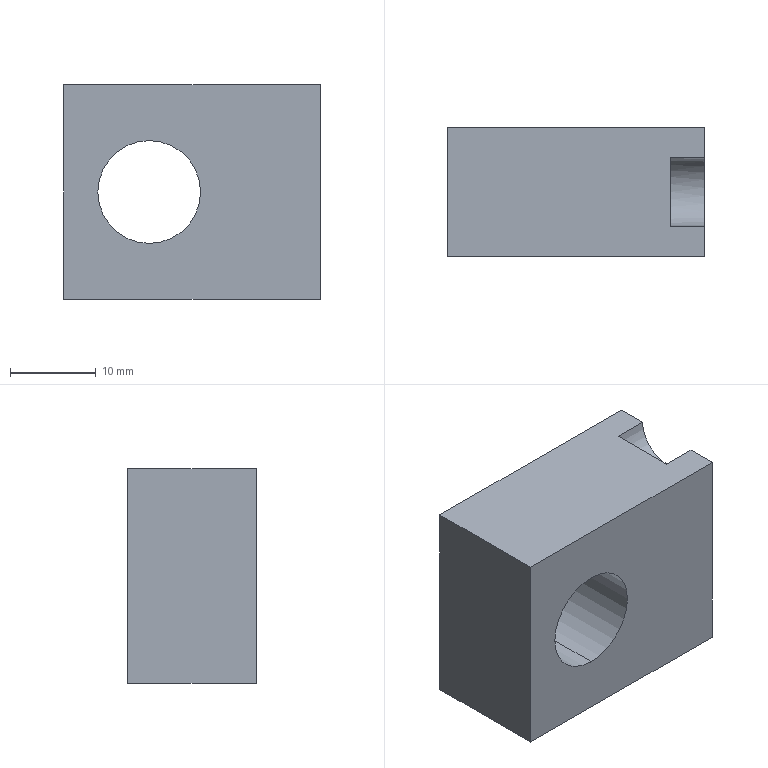Part | STEP file | Positioning_id1606_x_t | 1 solid | 13 faces | box 30 x 15 x 25 mm | volume 9340 mm3 | plane 8 | cylinder 5 | commonest cylinder face diameters 6 x2 12 x2 8 x1
STEP:
#1=CARTESIAN_POINT('',(0.,0.,0.));
#2=DIRECTION('',(0.,0.,1.));
#3=DIRECTION('',(1.,0.,0.));
#4=AXIS2_PLACEMENT_3D('',#1,#2,#3);
#5=CARTESIAN_POINT('',(-751.002,-201.5,188.032));
#6=VERTEX_POINT('',#5);
#7=CARTESIAN_POINT('',(-751.002,-201.5,194.032));
#8=VERTEX_POINT('',#7);
#9=CARTESIAN_POINT('',(-751.002,-201.5,191.032));
#10=DIRECTION('',(1.,0.,0.));
#11=DIRECTION('',(0.,0.,-1.));
#12=AXIS2_PLACEMENT_3D('',#9,#10,#11);
#13=CIRCLE('',#12,3.);
#14=CARTESIAN_POINT('',(-701.002,-201.5,191.032));
#15=DIRECTION('',(1.,0.,0.));
#16=DIRECTION('',(0.,0.,-1.));
#17=AXIS2_PLACEMENT_3D('',#14,#15,#16);
#18=CYLINDRICAL_SURFACE('',#17,3.);
#19=CARTESIAN_POINT('',(0.,-50.));
#20=DIRECTION('',(1.,0.));
#21=VECTOR('',#20,1.);
#22=LINE('',#19,#21);
#23=(GEOMETRIC_REPRESENTATION_CONTEXT(2)PARAMETRIC_REPRESENTATION_CONTEXT()REPRESENTATION_CONTEXT('',''));
#24=DEFINITIONAL_REPRESENTATION('',(#22),#23);
#25=PCURVE('',#18,#24);
#26=CARTESIAN_POINT('',(-751.002,-201.5,191.032));
#27=DIRECTION('',(-1.,0.,0.));
#28=DIRECTION('',(0.,0.,-1.));
#29=AXIS2_PLACEMENT_3D('',#26,#27,#28);
#30=PLANE('',#29);
#31=CARTESIAN_POINT('',(3.,0.));
#32=CARTESIAN_POINT('',(3.,-5.196));
#33=CARTESIAN_POINT('',(-1.5,-2.598));
#34=CARTESIAN_POINT('',(-6.,0.));
#35=CARTESIAN_POINT('',(-1.5,2.598));
#36=CARTESIAN_POINT('',(3.,5.196));
#37=CARTESIAN_POINT('',(3.,0.));
#38=(BOUNDED_CURVE()B_SPLINE_CURVE(2,(#31,#32,#33,#34,#35,#36,#37),.UNSPECIFIED.,.T.,.F.)B_SPLINE_CURVE_WITH_KNOTS((1,2,2,2,2,1),(-2.094,0.,2.094,4.189,6.283,8.378),.UNSPECIFIED.)CURVE()GEOMETRIC_REPRESENTATION_ITEM()RATIONAL_B_SPLINE_CURVE((1.,0.5,1.,0.5,1.,0.5,1.))REPRESENTATION_ITEM(''));
#39=(GEOMETRIC_REPRESENTATION_CONTEXT(2)PARAMETRIC_REPRESENTATION_CONTEXT()REPRESENTATION_CONTEXT('',''));
#40=DEFINITIONAL_REPRESENTATION('',(#38),#39);
#41=PCURVE('',#30,#40);
#42=SURFACE_CURVE('',#13,(#25,#41),.PCURVE_S1.);
#43=EDGE_CURVE('',#6,#8,#42,.T.);
#44=ORIENTED_EDGE('',*,*,#43,.T.);
#45=CARTESIAN_POINT('',(-747.002,-201.5,194.032));
#46=VERTEX_POINT('',#45);
#47=CARTESIAN_POINT('',(-747.002,-201.5,194.032));
#48=DIRECTION('',(1.,0.,0.));
#49=VECTOR('',#48,1.);
#50=LINE('',#47,#49);
#51=CARTESIAN_POINT('',(3.142,-46.));
#52=DIRECTION('',(0.,1.));
#53=VECTOR('',#52,1.);
#54=LINE('',#51,#53);
#55=(GEOMETRIC_REPRESENTATION_CONTEXT(2)PARAMETRIC_REPRESENTATION_CONTEXT()REPRESENTATION_CONTEXT('',''));
#56=DEFINITIONAL_REPRESENTATION('',(#54),#55);
#57=PCURVE('',#18,#56);
#58=CARTESIAN_POINT('',(-701.002,-201.5,191.032));
#59=DIRECTION('',(1.,0.,0.));
#60=DIRECTION('',(0.,0.,-1.));
#61=AXIS2_PLACEMENT_3D('',#58,#59,#60);
#62=CYLINDRICAL_SURFACE('',#61,3.);
#63=CARTESIAN_POINT('',(3.142,-46.));
#64=DIRECTION('',(0.,1.));
#65=VECTOR('',#64,1.);
#66=LINE('',#63,#65);
#67=(GEOMETRIC_REPRESENTATION_CONTEXT(2)PARAMETRIC_REPRESENTATION_CONTEXT()REPRESENTATION_CONTEXT('',''));
#68=DEFINITIONAL_REPRESENTATION('',(#66),#67);
#69=PCURVE('',#62,#68);
#70=SURFACE_CURVE('',#50,(#57,#69),.PCURVE_S1.);
#71=EDGE_CURVE('',#8,#46,#70,.T.);
#72=ORIENTED_EDGE('',*,*,#71,.T.);
#73=CARTESIAN_POINT('',(-747.002,-201.5,188.032));
#74=VERTEX_POINT('',#73);
#75=CARTESIAN_POINT('',(-747.002,-201.5,191.032));
#76=DIRECTION('',(-1.,0.,0.));
#77=DIRECTION('',(0.,0.,-1.));
#78=AXIS2_PLACEMENT_3D('',#75,#76,#77);
#79=CIRCLE('',#78,3.);
#80=CARTESIAN_POINT('',(6.283,-46.));
#81=DIRECTION('',(-1.,0.));
#82=VECTOR('',#81,1.);
#83=LINE('',#80,#82);
#84=(GEOMETRIC_REPRESENTATION_CONTEXT(2)PARAMETRIC_REPRESENTATION_CONTEXT()REPRESENTATION_CONTEXT('',''));
#85=DEFINITIONAL_REPRESENTATION('',(#83),#84);
#86=PCURVE('',#18,#85);
#87=CARTESIAN_POINT('',(-747.002,-194.,206.032));
#88=DIRECTION('',(1.,0.,0.));
#89=DIRECTION('',(0.,0.,-1.));
#90=AXIS2_PLACEMENT_3D('',#87,#88,#89);
#91=PLANE('',#90);
#92=CARTESIAN_POINT('',(18.,-7.5));
#93=CARTESIAN_POINT('',(18.,-12.696));
#94=CARTESIAN_POINT('',(13.5,-10.098));
#95=CARTESIAN_POINT('',(9.,-7.5));
#96=CARTESIAN_POINT('',(13.5,-4.902));
#97=CARTESIAN_POINT('',(18.,-2.304));
#98=CARTESIAN_POINT('',(18.,-7.5));
#99=(BOUNDED_CURVE()B_SPLINE_CURVE(2,(#92,#93,#94,#95,#96,#97,#98),.UNSPECIFIED.,.T.,.F.)B_SPLINE_CURVE_WITH_KNOTS((1,2,2,2,2,1),(-2.094,0.,2.094,4.189,6.283,8.378),.UNSPECIFIED.)CURVE()GEOMETRIC_REPRESENTATION_ITEM()RATIONAL_B_SPLINE_CURVE((1.,0.5,1.,0.5,1.,0.5,1.))REPRESENTATION_ITEM(''));
#100=(GEOMETRIC_REPRESENTATION_CONTEXT(2)PARAMETRIC_REPRESENTATION_CONTEXT()REPRESENTATION_CONTEXT('',''));
#101=DEFINITIONAL_REPRESENTATION('',(#99),#100);
#102=PCURVE('',#91,#101);
#103=SURFACE_CURVE('',#79,(#86,#102),.PCURVE_S1.);
#104=EDGE_CURVE('',#46,#74,#103,.T.);
#105=ORIENTED_EDGE('',*,*,#104,.T.);
#106=CARTESIAN_POINT('',(-747.002,-201.5,188.032));
#107=DIRECTION('',(-1.,0.,0.));
#108=VECTOR('',#107,1.);
#109=LINE('',#106,#108);
#110=CARTESIAN_POINT('',(0.,-46.));
#111=DIRECTION('',(0.,-1.));
#112=VECTOR('',#111,1.);
#113=LINE('',#110,#112);
#114=(GEOMETRIC_REPRESENTATION_CONTEXT(2)PARAMETRIC_REPRESENTATION_CONTEXT()REPRESENTATION_CONTEXT('',''));
#115=DEFINITIONAL_REPRESENTATION('',(#113),#114);
#116=PCURVE('',#18,#115);
#117=CARTESIAN_POINT('',(6.283,-46.));
#118=DIRECTION('',(0.,-1.));
#119=VECTOR('',#118,1.);
#120=LINE('',#117,#119);
#121=(GEOMETRIC_REPRESENTATION_CONTEXT(2)PARAMETRIC_REPRESENTATION_CONTEXT()REPRESENTATION_CONTEXT('',''));
#122=DEFINITIONAL_REPRESENTATION('',(#120),#121);
#123=PCURVE('',#62,#122);
#124=SURFACE_CURVE('',#109,(#116,#123),.PCURVE_S1.);
#125=EDGE_CURVE('',#74,#6,#124,.T.);
#126=ORIENTED_EDGE('',*,*,#125,.T.);
#127=EDGE_LOOP('',(#44,#72,#105,#126));
#128=FACE_BOUND('',#127,.F.);
#129=ADVANCED_FACE('',(#128),#18,.F.);
#130=CARTESIAN_POINT('',(-751.002,-201.5,194.032));
#131=CARTESIAN_POINT('',(-751.002,-204.5,194.032));
#132=CARTESIAN_POINT('',(-751.002,-206.,191.032));
#133=CARTESIAN_POINT('',(-751.002,-204.5,188.032));
#134=CARTESIAN_POINT('',(-751.002,-201.5,188.032));
#135=(BOUNDED_CURVE()B_SPLINE_CURVE(4,(#130,#131,#132,#133,#134),.UNSPECIFIED.,.F.,.F.)B_SPLINE_CURVE_WITH_KNOTS((5,5),(0.,1.),.PIECEWISE_BEZIER_KNOTS.)CURVE()GEOMETRIC_REPRESENTATION_ITEM()RATIONAL_B_SPLINE_CURVE((1.,0.7071,0.6667,0.7071,1.))REPRESENTATION_ITEM(''));
#136=CARTESIAN_POINT('',(-3.,0.));
#137=CARTESIAN_POINT('',(-3.,3.));
#138=CARTESIAN_POINT('',(0.,4.5));
#139=CARTESIAN_POINT('',(3.,3.));
#140=CARTESIAN_POINT('',(3.,0.));
#141=(BOUNDED_CURVE()B_SPLINE_CURVE(4,(#136,#137,#138,#139,#140),.UNSPECIFIED.,.F.,.F.)B_SPLINE_CURVE_WITH_KNOTS((5,5),(0.,1.),.PIECEWISE_BEZIER_KNOTS.)CURVE()GEOMETRIC_REPRESENTATION_ITEM()RATIONAL_B_SPLINE_CURVE((1.,0.7071,0.6667,0.7071,1.))REPRESENTATION_ITEM(''));
#142=(GEOMETRIC_REPRESENTATION_CONTEXT(2)PARAMETRIC_REPRESENTATION_CONTEXT()REPRESENTATION_CONTEXT('',''));
#143=DEFINITIONAL_REPRESENTATION('',(#141),#142);
#144=PCURVE('',#30,#143);
#145=CARTESIAN_POINT('',(3.142,-50.));
#146=CARTESIAN_POINT('',(3.184,-50.));
#147=CARTESIAN_POINT('',(3.271,-50.));
#148=CARTESIAN_POINT('',(3.405,-50.));
#149=CARTESIAN_POINT('',(3.542,-50.));
#150=CARTESIAN_POINT('',(3.681,-50.));
#151=CARTESIAN_POINT('',(3.823,-50.));
#152=CARTESIAN_POINT('',(3.968,-50.));
#153=CARTESIAN_POINT('',(4.114,-50.));
#154=CARTESIAN_POINT('',(4.262,-50.));
#155=CARTESIAN_POINT('',(4.412,-50.));
#156=CARTESIAN_POINT('',(4.562,-50.));
#157=CARTESIAN_POINT('',(4.712,-50.));
#158=CARTESIAN_POINT('',(4.863,-50.));
#159=CARTESIAN_POINT('',(5.013,-50.));
#160=CARTESIAN_POINT('',(5.163,-50.));
#161=CARTESIAN_POINT('',(5.311,-50.));
#162=CARTESIAN_POINT('',(5.457,-50.));
#163=CARTESIAN_POINT('',(5.602,-50.));
#164=CARTESIAN_POINT('',(5.744,-50.));
#165=CARTESIAN_POINT('',(5.883,-50.));
#166=CARTESIAN_POINT('',(6.02,-50.));
#167=CARTESIAN_POINT('',(6.153,-50.));
#168=CARTESIAN_POINT('',(6.24,-50.));
#169=CARTESIAN_POINT('',(6.283,-50.));
#170=B_SPLINE_CURVE_WITH_KNOTS('',3,(#145,#146,#147,#148,#149,#150,#151,#152,#153,#154,#155,#156,#157,#158,#159,#160,#161,#162,#163,#164,#165,#166,#167,#168,#169),.UNSPECIFIED.,.F.,.F.,(4,1,1,1,1,1,1,1,1,1,1,1,1,1,1,1,1,1,1,1,1,1,4),(0.,0.04545,0.09091,0.1364,0.1818,0.2273,0.2727,0.3182,0.3636,0.4091,0.4545,0.5,0.5455,0.5909,0.6364,0.6818,0.7273,0.7727,0.8182,0.8636,0.9091,0.9545,1.),.QUASI_UNIFORM_KNOTS.);
#171=(GEOMETRIC_REPRESENTATION_CONTEXT(2)PARAMETRIC_REPRESENTATION_CONTEXT()REPRESENTATION_CONTEXT('',''));
#172=DEFINITIONAL_REPRESENTATION('',(#170),#171);
#173=PCURVE('',#62,#172);
#174=SURFACE_CURVE('',#135,(#144,#173),.PCURVE_S1.);
#175=EDGE_CURVE('',#8,#6,#174,.T.);
#176=ORIENTED_EDGE('',*,*,#175,.T.);
#177=ORIENTED_EDGE('',*,*,#43,.T.);
#178=EDGE_LOOP('',(#176,#177));
#179=FACE_BOUND('',#178,.T.);
#180=ADVANCED_FACE('',(#179),#30,.F.);
#181=CARTESIAN_POINT('',(-747.002,-194.,181.032));
#182=VERTEX_POINT('',#181);
#183=CARTESIAN_POINT('',(-777.002,-194.,181.032));
#184=VERTEX_POINT('',#183);
#185=CARTESIAN_POINT('',(-747.002,-194.,181.032));
#186=DIRECTION('',(-1.,0.,0.));
#187=VECTOR('',#186,1.);
#188=LINE('',#185,#187);
#189=CARTESIAN_POINT('',(-701.002,-191.5,181.032));
#190=DIRECTION('',(0.,0.,-1.));
#191=DIRECTION('',(0.,1.,0.));
#192=AXIS2_PLACEMENT_3D('',#189,#190,#191);
#193=PLANE('',#192);
#194=CARTESIAN_POINT('',(-2.5,-46.));
#195=DIRECTION('',(0.,-1.));
#196=VECTOR('',#195,1.);
#197=LINE('',#194,#196);
#198=(GEOMETRIC_REPRESENTATION_CONTEXT(2)PARAMETRIC_REPRESENTATION_CONTEXT()REPRESENTATION_CONTEXT('',''));
#199=DEFINITIONAL_REPRESENTATION('',(#197),#198);
#200=PCURVE('',#193,#199);
#201=CARTESIAN_POINT('',(-759.502,-194.,187.282));
#202=DIRECTION('',(0.,1.,0.));
#203=DIRECTION('',(1.,0.,0.));
#204=AXIS2_PLACEMENT_3D('',#201,#202,#203);
#205=PLANE('',#204);
#206=CARTESIAN_POINT('',(12.5,6.25));
#207=DIRECTION('',(-1.,0.));
#208=VECTOR('',#207,1.);
#209=LINE('',#206,#208);
#210=(GEOMETRIC_REPRESENTATION_CONTEXT(2)PARAMETRIC_REPRESENTATION_CONTEXT()REPRESENTATION_CONTEXT('',''));
#211=DEFINITIONAL_REPRESENTATION('',(#209),#210);
#212=PCURVE('',#205,#211);
#213=SURFACE_CURVE('',#188,(#200,#212),.PCURVE_S1.);
#214=EDGE_CURVE('',#182,#184,#213,.T.);
#215=ORIENTED_EDGE('',*,*,#214,.F.);
#216=CARTESIAN_POINT('',(-747.002,-209.,181.032));
#217=VERTEX_POINT('',#216);
#218=CARTESIAN_POINT('',(-747.002,-194.,181.032));
#219=DIRECTION('',(0.,-1.,0.));
#220=VECTOR('',#219,1.);
#221=LINE('',#218,#220);
#222=CARTESIAN_POINT('',(-2.5,-46.));
#223=DIRECTION('',(-1.,0.));
#224=VECTOR('',#223,1.);
#225=LINE('',#222,#224);
#226=(GEOMETRIC_REPRESENTATION_CONTEXT(2)PARAMETRIC_REPRESENTATION_CONTEXT()REPRESENTATION_CONTEXT('',''));
#227=DEFINITIONAL_REPRESENTATION('',(#225),#226);
#228=PCURVE('',#193,#227);
#229=CARTESIAN_POINT('',(25.,0.));
#230=DIRECTION('',(0.,-1.));
#231=VECTOR('',#230,1.);
#232=LINE('',#229,#231);
#233=(GEOMETRIC_REPRESENTATION_CONTEXT(2)PARAMETRIC_REPRESENTATION_CONTEXT()REPRESENTATION_CONTEXT('',''));
#234=DEFINITIONAL_REPRESENTATION('',(#232),#233);
#235=PCURVE('',#91,#234);
#236=SURFACE_CURVE('',#221,(#228,#235),.PCURVE_S1.);
#237=EDGE_CURVE('',#182,#217,#236,.T.);
#238=ORIENTED_EDGE('',*,*,#237,.T.);
#239=CARTESIAN_POINT('',(-777.002,-209.,181.032));
#240=VERTEX_POINT('',#239);
#241=CARTESIAN_POINT('',(-777.002,-209.,181.032));
#242=DIRECTION('',(1.,0.,0.));
#243=VECTOR('',#242,1.);
#244=LINE('',#241,#243);
#245=CARTESIAN_POINT('',(-17.5,-76.));
#246=DIRECTION('',(0.,1.));
#247=VECTOR('',#246,1.);
#248=LINE('',#245,#247);
#249=(GEOMETRIC_REPRESENTATION_CONTEXT(2)PARAMETRIC_REPRESENTATION_CONTEXT()REPRESENTATION_CONTEXT('',''));
#250=DEFINITIONAL_REPRESENTATION('',(#248),#249);
#251=PCURVE('',#193,#250);
#252=CARTESIAN_POINT('',(-759.502,-209.,187.282));
#253=DIRECTION('',(0.,-1.,0.));
#254=DIRECTION('',(-1.,0.,0.));
#255=AXIS2_PLACEMENT_3D('',#252,#253,#254);
#256=PLANE('',#255);
#257=CARTESIAN_POINT('',(17.5,6.25));
#258=DIRECTION('',(-1.,0.));
#259=VECTOR('',#258,1.);
#260=LINE('',#257,#259);
#261=(GEOMETRIC_REPRESENTATION_CONTEXT(2)PARAMETRIC_REPRESENTATION_CONTEXT()REPRESENTATION_CONTEXT('',''));
#262=DEFINITIONAL_REPRESENTATION('',(#260),#261);
#263=PCURVE('',#256,#262);
#264=SURFACE_CURVE('',#244,(#251,#263),.PCURVE_S1.);
#265=EDGE_CURVE('',#240,#217,#264,.T.);
#266=ORIENTED_EDGE('',*,*,#265,.F.);
#267=CARTESIAN_POINT('',(-777.002,-194.,181.032));
#268=DIRECTION('',(0.,-1.,0.));
#269=VECTOR('',#268,1.);
#270=LINE('',#267,#269);
#271=CARTESIAN_POINT('',(-2.5,-76.));
#272=DIRECTION('',(-1.,0.));
#273=VECTOR('',#272,1.);
#274=LINE('',#271,#273);
#275=(GEOMETRIC_REPRESENTATION_CONTEXT(2)PARAMETRIC_REPRESENTATION_CONTEXT()REPRESENTATION_CONTEXT('',''));
#276=DEFINITIONAL_REPRESENTATION('',(#274),#275);
#277=PCURVE('',#193,#276);
#278=CARTESIAN_POINT('',(-777.002,-201.5,187.282));
#279=DIRECTION('',(-1.,0.,0.));
#280=DIRECTION('',(0.,1.,0.));
#281=AXIS2_PLACEMENT_3D('',#278,#279,#280);
#282=PLANE('',#281);
#283=CARTESIAN_POINT('',(7.5,6.25));
#284=DIRECTION('',(-1.,0.));
#285=VECTOR('',#284,1.);
#286=LINE('',#283,#285);
#287=(GEOMETRIC_REPRESENTATION_CONTEXT(2)PARAMETRIC_REPRESENTATION_CONTEXT()REPRESENTATION_CONTEXT('',''));
#288=DEFINITIONAL_REPRESENTATION('',(#286),#287);
#289=PCURVE('',#282,#288);
#290=SURFACE_CURVE('',#270,(#277,#289),.PCURVE_S1.);
#291=EDGE_CURVE('',#184,#240,#290,.T.);
#292=ORIENTED_EDGE('',*,*,#291,.F.);
#293=EDGE_LOOP('',(#215,#238,#266,#292));
#294=FACE_BOUND('',#293,.T.);
#295=ADVANCED_FACE('',(#294),#193,.T.);
#296=CARTESIAN_POINT('',(-767.002,-209.,187.532));
#297=VERTEX_POINT('',#296);
#298=CARTESIAN_POINT('',(-767.002,-209.,199.532));
#299=VERTEX_POINT('',#298);
#300=CARTESIAN_POINT('',(-767.002,-209.,193.532));
#301=DIRECTION('',(0.,1.,0.));
#302=DIRECTION('',(0.,0.,-1.));
#303=AXIS2_PLACEMENT_3D('',#300,#301,#302);
#304=CIRCLE('',#303,6.);
#305=CARTESIAN_POINT('',(7.5,-0.25));
#306=CARTESIAN_POINT('',(17.892,-0.25));
#307=CARTESIAN_POINT('',(12.696,-9.25));
#308=CARTESIAN_POINT('',(7.5,-18.25));
#309=CARTESIAN_POINT('',(2.304,-9.25));
#310=CARTESIAN_POINT('',(-2.892,-0.25));
#311=CARTESIAN_POINT('',(7.5,-0.25));
#312=(BOUNDED_CURVE()B_SPLINE_CURVE(2,(#305,#306,#307,#308,#309,#310,#311),.UNSPECIFIED.,.T.,.F.)B_SPLINE_CURVE_WITH_KNOTS((1,2,2,2,2,1),(-2.094,0.,2.094,4.189,6.283,8.378),.UNSPECIFIED.)CURVE()GEOMETRIC_REPRESENTATION_ITEM()RATIONAL_B_SPLINE_CURVE((1.,0.5,1.,0.5,1.,0.5,1.))REPRESENTATION_ITEM(''));
#313=(GEOMETRIC_REPRESENTATION_CONTEXT(2)PARAMETRIC_REPRESENTATION_CONTEXT()REPRESENTATION_CONTEXT('',''));
#314=DEFINITIONAL_REPRESENTATION('',(#312),#313);
#315=PCURVE('',#256,#314);
#316=CARTESIAN_POINT('',(-767.002,-214.,193.532));
#317=DIRECTION('',(0.,-1.,0.));
#318=DIRECTION('',(0.,0.,1.));
#319=AXIS2_PLACEMENT_3D('',#316,#317,#318);
#320=CYLINDRICAL_SURFACE('',#319,6.);
#321=CARTESIAN_POINT('',(3.142,-5.));
#322=DIRECTION('',(-1.,0.));
#323=VECTOR('',#322,1.);
#324=LINE('',#321,#323);
#325=(GEOMETRIC_REPRESENTATION_CONTEXT(2)PARAMETRIC_REPRESENTATION_CONTEXT()REPRESENTATION_CONTEXT('',''));
#326=DEFINITIONAL_REPRESENTATION('',(#324),#325);
#327=PCURVE('',#320,#326);
#328=SURFACE_CURVE('',#304,(#315,#327),.PCURVE_S1.);
#329=EDGE_CURVE('',#297,#299,#328,.T.);
#330=ORIENTED_EDGE('',*,*,#329,.T.);
#331=CARTESIAN_POINT('',(-767.002,-209.,193.532));
#332=DIRECTION('',(0.,1.,0.));
#333=DIRECTION('',(0.,0.,1.));
#334=AXIS2_PLACEMENT_3D('',#331,#332,#333);
#335=CIRCLE('',#334,6.);
#336=CARTESIAN_POINT('',(7.5,-12.25));
#337=CARTESIAN_POINT('',(-2.892,-12.25));
#338=CARTESIAN_POINT('',(2.304,-3.25));
#339=CARTESIAN_POINT('',(7.5,5.75));
#340=CARTESIAN_POINT('',(12.696,-3.25));
#341=CARTESIAN_POINT('',(17.892,-12.25));
#342=CARTESIAN_POINT('',(7.5,-12.25));
#343=(BOUNDED_CURVE()B_SPLINE_CURVE(2,(#336,#337,#338,#339,#340,#341,#342),.UNSPECIFIED.,.T.,.F.)B_SPLINE_CURVE_WITH_KNOTS((1,2,2,2,2,1),(-2.094,0.,2.094,4.189,6.283,8.378),.UNSPECIFIED.)CURVE()GEOMETRIC_REPRESENTATION_ITEM()RATIONAL_B_SPLINE_CURVE((1.,0.5,1.,0.5,1.,0.5,1.))REPRESENTATION_ITEM(''));
#344=(GEOMETRIC_REPRESENTATION_CONTEXT(2)PARAMETRIC_REPRESENTATION_CONTEXT()REPRESENTATION_CONTEXT('',''));
#345=DEFINITIONAL_REPRESENTATION('',(#343),#344);
#346=PCURVE('',#256,#345);
#347=CARTESIAN_POINT('',(-767.002,-214.,193.532));
#348=DIRECTION('',(0.,-1.,0.));
#349=DIRECTION('',(0.,0.,1.));
#350=AXIS2_PLACEMENT_3D('',#347,#348,#349);
#351=CYLINDRICAL_SURFACE('',#350,6.);
#352=CARTESIAN_POINT('',(6.283,-5.));
#353=DIRECTION('',(-1.,0.));
#354=VECTOR('',#353,1.);
#355=LINE('',#352,#354);
#356=(GEOMETRIC_REPRESENTATION_CONTEXT(2)PARAMETRIC_REPRESENTATION_CONTEXT()REPRESENTATION_CONTEXT('',''));
#357=DEFINITIONAL_REPRESENTATION('',(#355),#356);
#358=PCURVE('',#351,#357);
#359=SURFACE_CURVE('',#335,(#346,#358),.PCURVE_S1.);
#360=EDGE_CURVE('',#299,#297,#359,.T.);
#361=ORIENTED_EDGE('',*,*,#360,.T.);
#362=EDGE_LOOP('',(#330,#361));
#363=FACE_BOUND('',#362,.T.);
#364=CARTESIAN_POINT('',(-747.002,-209.,206.032));
#365=VERTEX_POINT('',#364);
#366=CARTESIAN_POINT('',(-777.002,-209.,206.032));
#367=VERTEX_POINT('',#366);
#368=CARTESIAN_POINT('',(-747.002,-209.,206.032));
#369=DIRECTION('',(-1.,0.,0.));
#370=VECTOR('',#369,1.);
#371=LINE('',#368,#370);
#372=CARTESIAN_POINT('',(-12.5,-18.75));
#373=DIRECTION('',(1.,0.));
#374=VECTOR('',#373,1.);
#375=LINE('',#372,#374);
#376=(GEOMETRIC_REPRESENTATION_CONTEXT(2)PARAMETRIC_REPRESENTATION_CONTEXT()REPRESENTATION_CONTEXT('',''));
#377=DEFINITIONAL_REPRESENTATION('',(#375),#376);
#378=PCURVE('',#256,#377);
#379=CARTESIAN_POINT('',(-759.502,-201.5,206.032));
#380=DIRECTION('',(0.,0.,1.));
#381=DIRECTION('',(0.,-1.,0.));
#382=AXIS2_PLACEMENT_3D('',#379,#380,#381);
#383=PLANE('',#382);
#384=CARTESIAN_POINT('',(7.5,12.5));
#385=DIRECTION('',(0.,-1.));
#386=VECTOR('',#385,1.);
#387=LINE('',#384,#386);
#388=(GEOMETRIC_REPRESENTATION_CONTEXT(2)PARAMETRIC_REPRESENTATION_CONTEXT()REPRESENTATION_CONTEXT('',''));
#389=DEFINITIONAL_REPRESENTATION('',(#387),#388);
#390=PCURVE('',#383,#389);
#391=SURFACE_CURVE('',#371,(#378,#390),.PCURVE_S1.);
#392=EDGE_CURVE('',#365,#367,#391,.T.);
#393=ORIENTED_EDGE('',*,*,#392,.T.);
#394=CARTESIAN_POINT('',(-777.002,-209.,206.032));
#395=DIRECTION('',(0.,0.,-1.));
#396=VECTOR('',#395,1.);
#397=LINE('',#394,#396);
#398=CARTESIAN_POINT('',(17.5,-18.75));
#399=DIRECTION('',(0.,1.));
#400=VECTOR('',#399,1.);
#401=LINE('',#398,#400);
#402=(GEOMETRIC_REPRESENTATION_CONTEXT(2)PARAMETRIC_REPRESENTATION_CONTEXT()REPRESENTATION_CONTEXT('',''));
#403=DEFINITIONAL_REPRESENTATION('',(#401),#402);
#404=PCURVE('',#256,#403);
#405=CARTESIAN_POINT('',(-7.5,-18.75));
#406=DIRECTION('',(0.,1.));
#407=VECTOR('',#406,1.);
#408=LINE('',#405,#407);
#409=(GEOMETRIC_REPRESENTATION_CONTEXT(2)PARAMETRIC_REPRESENTATION_CONTEXT()REPRESENTATION_CONTEXT('',''));
#410=DEFINITIONAL_REPRESENTATION('',(#408),#409);
#411=PCURVE('',#282,#410);
#412=SURFACE_CURVE('',#397,(#404,#411),.PCURVE_S1.);
#413=EDGE_CURVE('',#367,#240,#412,.T.);
#414=ORIENTED_EDGE('',*,*,#413,.T.);
#415=ORIENTED_EDGE('',*,*,#265,.T.);
#416=CARTESIAN_POINT('',(-747.002,-209.,181.032));
#417=DIRECTION('',(0.,0.,1.));
#418=VECTOR('',#417,1.);
#419=LINE('',#416,#418);
#420=CARTESIAN_POINT('',(-12.5,6.25));
#421=DIRECTION('',(0.,-1.));
#422=VECTOR('',#421,1.);
#423=LINE('',#420,#422);
#424=(GEOMETRIC_REPRESENTATION_CONTEXT(2)PARAMETRIC_REPRESENTATION_CONTEXT()REPRESENTATION_CONTEXT('',''));
#425=DEFINITIONAL_REPRESENTATION('',(#423),#424);
#426=PCURVE('',#256,#425);
#427=CARTESIAN_POINT('',(25.,-15.));
#428=DIRECTION('',(-1.,0.));
#429=VECTOR('',#428,1.);
#430=LINE('',#427,#429);
#431=(GEOMETRIC_REPRESENTATION_CONTEXT(2)PARAMETRIC_REPRESENTATION_CONTEXT()REPRESENTATION_CONTEXT('',''));
#432=DEFINITIONAL_REPRESENTATION('',(#430),#431);
#433=PCURVE('',#91,#432);
#434=SURFACE_CURVE('',#419,(#426,#433),.PCURVE_S1.);
#435=EDGE_CURVE('',#217,#365,#434,.T.);
#436=ORIENTED_EDGE('',*,*,#435,.T.);
#437=EDGE_LOOP('',(#393,#414,#415,#436));
#438=FACE_BOUND('',#437,.T.);
#439=ADVANCED_FACE('',(#363,#438),#256,.T.);
#440=CARTESIAN_POINT('',(-747.002,-197.5,206.032));
#441=VERTEX_POINT('',#440);
#442=CARTESIAN_POINT('',(-751.002,-197.5,206.032));
#443=VERTEX_POINT('',#442);
#444=CARTESIAN_POINT('',(-747.002,-197.5,206.032));
#445=DIRECTION('',(-1.,0.,0.));
#446=VECTOR('',#445,1.);
#447=LINE('',#444,#446);
#448=CARTESIAN_POINT('',(-4.,12.5));
#449=DIRECTION('',(0.,-1.));
#450=VECTOR('',#449,1.);
#451=LINE('',#448,#450);
#452=(GEOMETRIC_REPRESENTATION_CONTEXT(2)PARAMETRIC_REPRESENTATION_CONTEXT()REPRESENTATION_CONTEXT('',''));
#453=DEFINITIONAL_REPRESENTATION('',(#451),#452);
#454=PCURVE('',#383,#453);
#455=CARTESIAN_POINT('',(-701.002,-201.5,206.032));
#456=DIRECTION('',(1.,0.,0.));
#457=DIRECTION('',(0.,0.,-1.));
#458=AXIS2_PLACEMENT_3D('',#455,#456,#457);
#459=CYLINDRICAL_SURFACE('',#458,4.);
#460=CARTESIAN_POINT('',(7.854,-46.));
#461=DIRECTION('',(0.,-1.));
#462=VECTOR('',#461,1.);
#463=LINE('',#460,#462);
#464=(GEOMETRIC_REPRESENTATION_CONTEXT(2)PARAMETRIC_REPRESENTATION_CONTEXT()REPRESENTATION_CONTEXT('',''));
#465=DEFINITIONAL_REPRESENTATION('',(#463),#464);
#466=PCURVE('',#459,#465);
#467=SURFACE_CURVE('',#447,(#454,#466),.PCURVE_S1.);
#468=EDGE_CURVE('',#441,#443,#467,.T.);
#469=ORIENTED_EDGE('',*,*,#468,.F.);
#470=CARTESIAN_POINT('',(-747.002,-194.,206.032));
#471=VERTEX_POINT('',#470);
#472=CARTESIAN_POINT('',(-747.002,-194.,206.032));
#473=DIRECTION('',(0.,-1.,0.));
#474=VECTOR('',#473,1.);
#475=LINE('',#472,#474);
#476=CARTESIAN_POINT('',(-7.5,12.5));
#477=DIRECTION('',(1.,0.));
#478=VECTOR('',#477,1.);
#479=LINE('',#476,#478);
#480=(GEOMETRIC_REPRESENTATION_CONTEXT(2)PARAMETRIC_REPRESENTATION_CONTEXT()REPRESENTATION_CONTEXT('',''));
#481=DEFINITIONAL_REPRESENTATION('',(#479),#480);
#482=PCURVE('',#383,#481);
#483=CARTESIAN_POINT('',(0.,0.));
#484=DIRECTION('',(0.,-1.));
#485=VECTOR('',#484,1.);
#486=LINE('',#483,#485);
#487=(GEOMETRIC_REPRESENTATION_CONTEXT(2)PARAMETRIC_REPRESENTATION_CONTEXT()REPRESENTATION_CONTEXT('',''));
#488=DEFINITIONAL_REPRESENTATION('',(#486),#487);
#489=PCURVE('',#91,#488);
#490=SURFACE_CURVE('',#475,(#482,#489),.PCURVE_S1.);
#491=EDGE_CURVE('',#471,#441,#490,.T.);
#492=ORIENTED_EDGE('',*,*,#491,.F.);
#493=CARTESIAN_POINT('',(-777.002,-194.,206.032));
#494=VERTEX_POINT('',#493);
#495=CARTESIAN_POINT('',(-777.002,-194.,206.032));
#496=DIRECTION('',(1.,0.,0.));
#497=VECTOR('',#496,1.);
#498=LINE('',#495,#497);
#499=CARTESIAN_POINT('',(-7.5,-17.5));
#500=DIRECTION('',(0.,1.));
#501=VECTOR('',#500,1.);
#502=LINE('',#499,#501);
#503=(GEOMETRIC_REPRESENTATION_CONTEXT(2)PARAMETRIC_REPRESENTATION_CONTEXT()REPRESENTATION_CONTEXT('',''));
#504=DEFINITIONAL_REPRESENTATION('',(#502),#503);
#505=PCURVE('',#383,#504);
#506=CARTESIAN_POINT('',(-17.5,-18.75));
#507=DIRECTION('',(1.,0.));
#508=VECTOR('',#507,1.);
#509=LINE('',#506,#508);
#510=(GEOMETRIC_REPRESENTATION_CONTEXT(2)PARAMETRIC_REPRESENTATION_CONTEXT()REPRESENTATION_CONTEXT('',''));
#511=DEFINITIONAL_REPRESENTATION('',(#509),#510);
#512=PCURVE('',#205,#511);
#513=SURFACE_CURVE('',#498,(#505,#512),.PCURVE_S1.);
#514=EDGE_CURVE('',#494,#471,#513,.T.);
#515=ORIENTED_EDGE('',*,*,#514,.F.);
#516=CARTESIAN_POINT('',(-777.002,-194.,206.032));
#517=DIRECTION('',(0.,-1.,0.));
#518=VECTOR('',#517,1.);
#519=LINE('',#516,#518);
#520=CARTESIAN_POINT('',(-7.5,-17.5));
#521=DIRECTION('',(1.,0.));
#522=VECTOR('',#521,1.);
#523=LINE('',#520,#522);
#524=(GEOMETRIC_REPRESENTATION_CONTEXT(2)PARAMETRIC_REPRESENTATION_CONTEXT()REPRESENTATION_CONTEXT('',''));
#525=DEFINITIONAL_REPRESENTATION('',(#523),#524);
#526=PCURVE('',#383,#525);
#527=CARTESIAN_POINT('',(7.5,-18.75));
#528=DIRECTION('',(-1.,0.));
#529=VECTOR('',#528,1.);
#530=LINE('',#527,#529);
#531=(GEOMETRIC_REPRESENTATION_CONTEXT(2)PARAMETRIC_REPRESENTATION_CONTEXT()REPRESENTATION_CONTEXT('',''));
#532=DEFINITIONAL_REPRESENTATION('',(#530),#531);
#533=PCURVE('',#282,#532);
#534=SURFACE_CURVE('',#519,(#526,#533),.PCURVE_S1.);
#535=EDGE_CURVE('',#494,#367,#534,.T.);
#536=ORIENTED_EDGE('',*,*,#535,.T.);
#537=ORIENTED_EDGE('',*,*,#392,.F.);
#538=CARTESIAN_POINT('',(-747.002,-205.5,206.032));
#539=VERTEX_POINT('',#538);
#540=CARTESIAN_POINT('',(-747.002,-205.5,206.032));
#541=DIRECTION('',(0.,-1.,0.));
#542=VECTOR('',#541,1.);
#543=LINE('',#540,#542);
#544=CARTESIAN_POINT('',(4.,12.5));
#545=DIRECTION('',(1.,0.));
#546=VECTOR('',#545,1.);
#547=LINE('',#544,#546);
#548=(GEOMETRIC_REPRESENTATION_CONTEXT(2)PARAMETRIC_REPRESENTATION_CONTEXT()REPRESENTATION_CONTEXT('',''));
#549=DEFINITIONAL_REPRESENTATION('',(#547),#548);
#550=PCURVE('',#383,#549);
#551=CARTESIAN_POINT('',(0.,-11.5));
#552=DIRECTION('',(0.,-1.));
#553=VECTOR('',#552,1.);
#554=LINE('',#551,#553);
#555=(GEOMETRIC_REPRESENTATION_CONTEXT(2)PARAMETRIC_REPRESENTATION_CONTEXT()REPRESENTATION_CONTEXT('',''));
#556=DEFINITIONAL_REPRESENTATION('',(#554),#555);
#557=PCURVE('',#91,#556);
#558=SURFACE_CURVE('',#543,(#550,#557),.PCURVE_S1.);
#559=EDGE_CURVE('',#539,#365,#558,.T.);
#560=ORIENTED_EDGE('',*,*,#559,.F.);
#561=CARTESIAN_POINT('',(-751.002,-205.5,206.032));
#562=VERTEX_POINT('',#561);
#563=CARTESIAN_POINT('',(-751.002,-205.5,206.032));
#564=DIRECTION('',(1.,0.,0.));
#565=VECTOR('',#564,1.);
#566=LINE('',#563,#565);
#567=CARTESIAN_POINT('',(4.,8.5));
#568=DIRECTION('',(0.,1.));
#569=VECTOR('',#568,1.);
#570=LINE('',#567,#569);
#571=(GEOMETRIC_REPRESENTATION_CONTEXT(2)PARAMETRIC_REPRESENTATION_CONTEXT()REPRESENTATION_CONTEXT('',''));
#572=DEFINITIONAL_REPRESENTATION('',(#570),#571);
#573=PCURVE('',#383,#572);
#574=CARTESIAN_POINT('',(4.712,-50.));
#575=DIRECTION('',(0.,1.));
#576=VECTOR('',#575,1.);
#577=LINE('',#574,#576);
#578=(GEOMETRIC_REPRESENTATION_CONTEXT(2)PARAMETRIC_REPRESENTATION_CONTEXT()REPRESENTATION_CONTEXT('',''));
#579=DEFINITIONAL_REPRESENTATION('',(#577),#578);
#580=PCURVE('',#459,#579);
#581=SURFACE_CURVE('',#566,(#573,#580),.PCURVE_S1.);
#582=EDGE_CURVE('',#562,#539,#581,.T.);
#583=ORIENTED_EDGE('',*,*,#582,.F.);
#584=CARTESIAN_POINT('',(-751.002,-197.5,206.032));
#585=DIRECTION('',(0.,-1.,0.));
#586=VECTOR('',#585,1.);
#587=LINE('',#584,#586);
#588=CARTESIAN_POINT('',(-4.,8.5));
#589=DIRECTION('',(1.,0.));
#590=VECTOR('',#589,1.);
#591=LINE('',#588,#590);
#592=(GEOMETRIC_REPRESENTATION_CONTEXT(2)PARAMETRIC_REPRESENTATION_CONTEXT()REPRESENTATION_CONTEXT('',''));
#593=DEFINITIONAL_REPRESENTATION('',(#591),#592);
#594=PCURVE('',#383,#593);
#595=CARTESIAN_POINT('',(-751.002,-201.5,206.032));
#596=DIRECTION('',(-1.,0.,0.));
#597=DIRECTION('',(0.,0.,-1.));
#598=AXIS2_PLACEMENT_3D('',#595,#596,#597);
#599=PLANE('',#598);
#600=CARTESIAN_POINT('',(0.,-4.));
#601=DIRECTION('',(0.,1.));
#602=VECTOR('',#601,1.);
#603=LINE('',#600,#602);
#604=(GEOMETRIC_REPRESENTATION_CONTEXT(2)PARAMETRIC_REPRESENTATION_CONTEXT()REPRESENTATION_CONTEXT('',''));
#605=DEFINITIONAL_REPRESENTATION('',(#603),#604);
#606=PCURVE('',#599,#605);
#607=SURFACE_CURVE('',#587,(#594,#606),.PCURVE_S1.);
#608=EDGE_CURVE('',#443,#562,#607,.T.);
#609=ORIENTED_EDGE('',*,*,#608,.F.);
#610=EDGE_LOOP('',(#469,#492,#515,#536,#537,#560,#583,#609));
#611=FACE_BOUND('',#610,.T.);
#612=ADVANCED_FACE('',(#611),#383,.T.);
#613=ORIENTED_EDGE('',*,*,#582,.F.);
#614=CARTESIAN_POINT('',(-751.002,-201.5,202.032));
#615=VERTEX_POINT('',#614);
#616=CARTESIAN_POINT('',(-751.002,-201.5,206.032));
#617=DIRECTION('',(1.,0.,0.));
#618=DIRECTION('',(0.,0.,-1.));
#619=AXIS2_PLACEMENT_3D('',#616,#617,#618);
#620=CIRCLE('',#619,4.);
#621=CARTESIAN_POINT('',(0.,-50.));
#622=DIRECTION('',(1.,0.));
#623=VECTOR('',#622,1.);
#624=LINE('',#621,#623);
#625=(GEOMETRIC_REPRESENTATION_CONTEXT(2)PARAMETRIC_REPRESENTATION_CONTEXT()REPRESENTATION_CONTEXT('',''));
#626=DEFINITIONAL_REPRESENTATION('',(#624),#625);
#627=PCURVE('',#459,#626);
#628=CARTESIAN_POINT('',(4.,0.));
#629=CARTESIAN_POINT('',(4.,-6.928));
#630=CARTESIAN_POINT('',(-2.,-3.464));
#631=CARTESIAN_POINT('',(-8.,0.));
#632=CARTESIAN_POINT('',(-2.,3.464));
#633=CARTESIAN_POINT('',(4.,6.928));
#634=CARTESIAN_POINT('',(4.,0.));
#635=(BOUNDED_CURVE()B_SPLINE_CURVE(2,(#628,#629,#630,#631,#632,#633,#634),.UNSPECIFIED.,.T.,.F.)B_SPLINE_CURVE_WITH_KNOTS((1,2,2,2,2,1),(-2.094,0.,2.094,4.189,6.283,8.378),.UNSPECIFIED.)CURVE()GEOMETRIC_REPRESENTATION_ITEM()RATIONAL_B_SPLINE_CURVE((1.,0.5,1.,0.5,1.,0.5,1.))REPRESENTATION_ITEM(''));
#636=(GEOMETRIC_REPRESENTATION_CONTEXT(2)PARAMETRIC_REPRESENTATION_CONTEXT()REPRESENTATION_CONTEXT('',''));
#637=DEFINITIONAL_REPRESENTATION('',(#635),#636);
#638=PCURVE('',#599,#637);
#639=SURFACE_CURVE('',#620,(#627,#638),.PCURVE_S1.);
#640=EDGE_CURVE('',#562,#615,#639,.T.);
#641=ORIENTED_EDGE('',*,*,#640,.T.);
#642=CARTESIAN_POINT('',(-751.002,-201.5,206.032));
#643=DIRECTION('',(1.,0.,0.));
#644=DIRECTION('',(0.,0.,-1.));
#645=AXIS2_PLACEMENT_3D('',#642,#643,#644);
#646=CIRCLE('',#645,4.);
#647=CARTESIAN_POINT('',(6.283,-50.));
#648=DIRECTION('',(1.,0.));
#649=VECTOR('',#648,1.);
#650=LINE('',#647,#649);
#651=(GEOMETRIC_REPRESENTATION_CONTEXT(2)PARAMETRIC_REPRESENTATION_CONTEXT()REPRESENTATION_CONTEXT('',''));
#652=DEFINITIONAL_REPRESENTATION('',(#650),#651);
#653=PCURVE('',#459,#652);
#654=CARTESIAN_POINT('',(4.,0.));
#655=CARTESIAN_POINT('',(4.,-6.928));
#656=CARTESIAN_POINT('',(-2.,-3.464));
#657=CARTESIAN_POINT('',(-8.,0.));
#658=CARTESIAN_POINT('',(-2.,3.464));
#659=CARTESIAN_POINT('',(4.,6.928));
#660=CARTESIAN_POINT('',(4.,0.));
#661=(BOUNDED_CURVE()B_SPLINE_CURVE(2,(#654,#655,#656,#657,#658,#659,#660),.UNSPECIFIED.,.T.,.F.)B_SPLINE_CURVE_WITH_KNOTS((1,2,2,2,2,1),(-2.094,0.,2.094,4.189,6.283,8.378),.UNSPECIFIED.)CURVE()GEOMETRIC_REPRESENTATION_ITEM()RATIONAL_B_SPLINE_CURVE((1.,0.5,1.,0.5,1.,0.5,1.))REPRESENTATION_ITEM(''));
#662=(GEOMETRIC_REPRESENTATION_CONTEXT(2)PARAMETRIC_REPRESENTATION_CONTEXT()REPRESENTATION_CONTEXT('',''));
#663=DEFINITIONAL_REPRESENTATION('',(#661),#662);
#664=PCURVE('',#599,#663);
#665=SURFACE_CURVE('',#646,(#653,#664),.PCURVE_S1.);
#666=EDGE_CURVE('',#615,#443,#665,.T.);
#667=ORIENTED_EDGE('',*,*,#666,.T.);
#668=ORIENTED_EDGE('',*,*,#468,.F.);
#669=CARTESIAN_POINT('',(-747.002,-201.5,206.032));
#670=DIRECTION('',(-1.,0.,0.));
#671=DIRECTION('',(0.,0.,-1.));
#672=AXIS2_PLACEMENT_3D('',#669,#670,#671);
#673=CIRCLE('',#672,4.);
#674=CARTESIAN_POINT('',(12.566,-46.));
#675=DIRECTION('',(-1.,0.));
#676=VECTOR('',#675,1.);
#677=LINE('',#674,#676);
#678=(GEOMETRIC_REPRESENTATION_CONTEXT(2)PARAMETRIC_REPRESENTATION_CONTEXT()REPRESENTATION_CONTEXT('',''));
#679=DEFINITIONAL_REPRESENTATION('',(#677),#678);
#680=PCURVE('',#459,#679);
#681=CARTESIAN_POINT('',(4.,-7.5));
#682=CARTESIAN_POINT('',(4.,-14.428));
#683=CARTESIAN_POINT('',(-2.,-10.964));
#684=CARTESIAN_POINT('',(-8.,-7.5));
#685=CARTESIAN_POINT('',(-2.,-4.036));
#686=CARTESIAN_POINT('',(4.,-0.5718));
#687=CARTESIAN_POINT('',(4.,-7.5));
#688=(BOUNDED_CURVE()B_SPLINE_CURVE(2,(#681,#682,#683,#684,#685,#686,#687),.UNSPECIFIED.,.T.,.F.)B_SPLINE_CURVE_WITH_KNOTS((1,2,2,2,2,1),(-2.094,0.,2.094,4.189,6.283,8.378),.UNSPECIFIED.)CURVE()GEOMETRIC_REPRESENTATION_ITEM()RATIONAL_B_SPLINE_CURVE((1.,0.5,1.,0.5,1.,0.5,1.))REPRESENTATION_ITEM(''));
#689=(GEOMETRIC_REPRESENTATION_CONTEXT(2)PARAMETRIC_REPRESENTATION_CONTEXT()REPRESENTATION_CONTEXT('',''));
#690=DEFINITIONAL_REPRESENTATION('',(#688),#689);
#691=PCURVE('',#91,#690);
#692=SURFACE_CURVE('',#673,(#680,#691),.PCURVE_S1.);
#693=EDGE_CURVE('',#441,#539,#692,.T.);
#694=ORIENTED_EDGE('',*,*,#693,.T.);
#695=EDGE_LOOP('',(#613,#641,#667,#668,#694));
#696=FACE_BOUND('',#695,.F.);
#697=ADVANCED_FACE('',(#696),#459,.F.);
#698=CARTESIAN_POINT('',(-767.002,-194.,187.532));
#699=VERTEX_POINT('',#698);
#700=CARTESIAN_POINT('',(-767.002,-194.,199.532));
#701=VERTEX_POINT('',#700);
#702=CARTESIAN_POINT('',(-767.002,-194.,193.532));
#703=DIRECTION('',(0.,-1.,0.));
#704=DIRECTION('',(0.,0.,-1.));
#705=AXIS2_PLACEMENT_3D('',#702,#703,#704);
#706=CIRCLE('',#705,6.);
#707=CARTESIAN_POINT('',(-7.5,-0.25));
#708=CARTESIAN_POINT('',(2.892,-0.25));
#709=CARTESIAN_POINT('',(-2.304,-9.25));
#710=CARTESIAN_POINT('',(-7.5,-18.25));
#711=CARTESIAN_POINT('',(-12.696,-9.25));
#712=CARTESIAN_POINT('',(-17.892,-0.25));
#713=CARTESIAN_POINT('',(-7.5,-0.25));
#714=(BOUNDED_CURVE()B_SPLINE_CURVE(2,(#707,#708,#709,#710,#711,#712,#713),.UNSPECIFIED.,.T.,.F.)B_SPLINE_CURVE_WITH_KNOTS((1,2,2,2,2,1),(-2.094,0.,2.094,4.189,6.283,8.378),.UNSPECIFIED.)CURVE()GEOMETRIC_REPRESENTATION_ITEM()RATIONAL_B_SPLINE_CURVE((1.,0.5,1.,0.5,1.,0.5,1.))REPRESENTATION_ITEM(''));
#715=(GEOMETRIC_REPRESENTATION_CONTEXT(2)PARAMETRIC_REPRESENTATION_CONTEXT()REPRESENTATION_CONTEXT('',''));
#716=DEFINITIONAL_REPRESENTATION('',(#714),#715);
#717=PCURVE('',#205,#716);
#718=CARTESIAN_POINT('',(3.142,-20.));
#719=DIRECTION('',(1.,0.));
#720=VECTOR('',#719,1.);
#721=LINE('',#718,#720);
#722=(GEOMETRIC_REPRESENTATION_CONTEXT(2)PARAMETRIC_REPRESENTATION_CONTEXT()REPRESENTATION_CONTEXT('',''));
#723=DEFINITIONAL_REPRESENTATION('',(#721),#722);
#724=PCURVE('',#351,#723);
#725=SURFACE_CURVE('',#706,(#717,#724),.PCURVE_S1.);
#726=EDGE_CURVE('',#699,#701,#725,.T.);
#727=ORIENTED_EDGE('',*,*,#726,.T.);
#728=CARTESIAN_POINT('',(-767.002,-194.,193.532));
#729=DIRECTION('',(0.,-1.,0.));
#730=DIRECTION('',(0.,0.,1.));
#731=AXIS2_PLACEMENT_3D('',#728,#729,#730);
#732=CIRCLE('',#731,6.);
#733=CARTESIAN_POINT('',(-7.5,-12.25));
#734=CARTESIAN_POINT('',(-17.892,-12.25));
#735=CARTESIAN_POINT('',(-12.696,-3.25));
#736=CARTESIAN_POINT('',(-7.5,5.75));
#737=CARTESIAN_POINT('',(-2.304,-3.25));
#738=CARTESIAN_POINT('',(2.892,-12.25));
#739=CARTESIAN_POINT('',(-7.5,-12.25));
#740=(BOUNDED_CURVE()B_SPLINE_CURVE(2,(#733,#734,#735,#736,#737,#738,#739),.UNSPECIFIED.,.T.,.F.)B_SPLINE_CURVE_WITH_KNOTS((1,2,2,2,2,1),(-2.094,0.,2.094,4.189,6.283,8.378),.UNSPECIFIED.)CURVE()GEOMETRIC_REPRESENTATION_ITEM()RATIONAL_B_SPLINE_CURVE((1.,0.5,1.,0.5,1.,0.5,1.))REPRESENTATION_ITEM(''));
#741=(GEOMETRIC_REPRESENTATION_CONTEXT(2)PARAMETRIC_REPRESENTATION_CONTEXT()REPRESENTATION_CONTEXT('',''));
#742=DEFINITIONAL_REPRESENTATION('',(#740),#741);
#743=PCURVE('',#205,#742);
#744=CARTESIAN_POINT('',(0.,-20.));
#745=DIRECTION('',(1.,0.));
#746=VECTOR('',#745,1.);
#747=LINE('',#744,#746);
#748=(GEOMETRIC_REPRESENTATION_CONTEXT(2)PARAMETRIC_REPRESENTATION_CONTEXT()REPRESENTATION_CONTEXT('',''));
#749=DEFINITIONAL_REPRESENTATION('',(#747),#748);
#750=PCURVE('',#320,#749);
#751=SURFACE_CURVE('',#732,(#743,#750),.PCURVE_S1.);
#752=EDGE_CURVE('',#701,#699,#751,.T.);
#753=ORIENTED_EDGE('',*,*,#752,.T.);
#754=EDGE_LOOP('',(#727,#753));
#755=FACE_BOUND('',#754,.T.);
#756=CARTESIAN_POINT('',(-747.002,-194.,206.032));
#757=DIRECTION('',(0.,0.,-1.));
#758=VECTOR('',#757,1.);
#759=LINE('',#756,#758);
#760=CARTESIAN_POINT('',(12.5,-18.75));
#761=DIRECTION('',(0.,1.));
#762=VECTOR('',#761,1.);
#763=LINE('',#760,#762);
#764=(GEOMETRIC_REPRESENTATION_CONTEXT(2)PARAMETRIC_REPRESENTATION_CONTEXT()REPRESENTATION_CONTEXT('',''));
#765=DEFINITIONAL_REPRESENTATION('',(#763),#764);
#766=PCURVE('',#205,#765);
#767=CARTESIAN_POINT('',(0.,0.));
#768=DIRECTION('',(1.,0.));
#769=VECTOR('',#768,1.);
#770=LINE('',#767,#769);
#771=(GEOMETRIC_REPRESENTATION_CONTEXT(2)PARAMETRIC_REPRESENTATION_CONTEXT()REPRESENTATION_CONTEXT('',''));
#772=DEFINITIONAL_REPRESENTATION('',(#770),#771);
#773=PCURVE('',#91,#772);
#774=SURFACE_CURVE('',#759,(#766,#773),.PCURVE_S1.);
#775=EDGE_CURVE('',#471,#182,#774,.T.);
#776=ORIENTED_EDGE('',*,*,#775,.T.);
#777=ORIENTED_EDGE('',*,*,#214,.T.);
#778=CARTESIAN_POINT('',(-777.002,-194.,181.032));
#779=DIRECTION('',(0.,0.,1.));
#780=VECTOR('',#779,1.);
#781=LINE('',#778,#780);
#782=CARTESIAN_POINT('',(-17.5,6.25));
#783=DIRECTION('',(0.,-1.));
#784=VECTOR('',#783,1.);
#785=LINE('',#782,#784);
#786=(GEOMETRIC_REPRESENTATION_CONTEXT(2)PARAMETRIC_REPRESENTATION_CONTEXT()REPRESENTATION_CONTEXT('',''));
#787=DEFINITIONAL_REPRESENTATION('',(#785),#786);
#788=PCURVE('',#205,#787);
#789=CARTESIAN_POINT('',(7.5,6.25));
#790=DIRECTION('',(0.,-1.));
#791=VECTOR('',#790,1.);
#792=LINE('',#789,#791);
#793=(GEOMETRIC_REPRESENTATION_CONTEXT(2)PARAMETRIC_REPRESENTATION_CONTEXT()REPRESENTATION_CONTEXT('',''));
#794=DEFINITIONAL_REPRESENTATION('',(#792),#793);
#795=PCURVE('',#282,#794);
#796=SURFACE_CURVE('',#781,(#788,#795),.PCURVE_S1.);
#797=EDGE_CURVE('',#184,#494,#796,.T.);
#798=ORIENTED_EDGE('',*,*,#797,.T.);
#799=ORIENTED_EDGE('',*,*,#514,.T.);
#800=EDGE_LOOP('',(#776,#777,#798,#799));
#801=FACE_BOUND('',#800,.T.);
#802=ADVANCED_FACE('',(#755,#801),#205,.T.);
#803=ORIENTED_EDGE('',*,*,#608,.T.);
#804=ORIENTED_EDGE('',*,*,#640,.T.);
#805=ORIENTED_EDGE('',*,*,#666,.T.);
#806=EDGE_LOOP('',(#803,#804,#805));
#807=FACE_BOUND('',#806,.T.);
#808=ADVANCED_FACE('',(#807),#599,.F.);
#809=ORIENTED_EDGE('',*,*,#752,.T.);
#810=CARTESIAN_POINT('',(-767.002,-209.,187.532));
#811=DIRECTION('',(0.,-1.,0.));
#812=VECTOR('',#811,1.);
#813=LINE('',#810,#812);
#814=CARTESIAN_POINT('',(3.142,-5.));
#815=DIRECTION('',(0.,1.));
#816=VECTOR('',#815,1.);
#817=LINE('',#814,#816);
#818=(GEOMETRIC_REPRESENTATION_CONTEXT(2)PARAMETRIC_REPRESENTATION_CONTEXT()REPRESENTATION_CONTEXT('',''));
#819=DEFINITIONAL_REPRESENTATION('',(#817),#818);
#820=PCURVE('',#320,#819);
#821=CARTESIAN_POINT('',(3.142,-5.));
#822=DIRECTION('',(0.,1.));
#823=VECTOR('',#822,1.);
#824=LINE('',#821,#823);
#825=(GEOMETRIC_REPRESENTATION_CONTEXT(2)PARAMETRIC_REPRESENTATION_CONTEXT()REPRESENTATION_CONTEXT('',''));
#826=DEFINITIONAL_REPRESENTATION('',(#824),#825);
#827=PCURVE('',#351,#826);
#828=SURFACE_CURVE('',#813,(#820,#827),.PCURVE_S1.);
#829=EDGE_CURVE('',#699,#297,#828,.T.);
#830=ORIENTED_EDGE('',*,*,#829,.T.);
#831=ORIENTED_EDGE('',*,*,#329,.T.);
#832=CARTESIAN_POINT('',(-767.002,-209.,199.532));
#833=DIRECTION('',(0.,1.,0.));
#834=VECTOR('',#833,1.);
#835=LINE('',#832,#834);
#836=CARTESIAN_POINT('',(0.,-5.));
#837=DIRECTION('',(0.,-1.));
#838=VECTOR('',#837,1.);
#839=LINE('',#836,#838);
#840=(GEOMETRIC_REPRESENTATION_CONTEXT(2)PARAMETRIC_REPRESENTATION_CONTEXT()REPRESENTATION_CONTEXT('',''));
#841=DEFINITIONAL_REPRESENTATION('',(#839),#840);
#842=PCURVE('',#320,#841);
#843=CARTESIAN_POINT('',(6.283,-5.));
#844=DIRECTION('',(0.,-1.));
#845=VECTOR('',#844,1.);
#846=LINE('',#843,#845);
#847=(GEOMETRIC_REPRESENTATION_CONTEXT(2)PARAMETRIC_REPRESENTATION_CONTEXT()REPRESENTATION_CONTEXT('',''));
#848=DEFINITIONAL_REPRESENTATION('',(#846),#847);
#849=PCURVE('',#351,#848);
#850=SURFACE_CURVE('',#835,(#842,#849),.PCURVE_S1.);
#851=EDGE_CURVE('',#299,#701,#850,.T.);
#852=ORIENTED_EDGE('',*,*,#851,.T.);
#853=EDGE_LOOP('',(#809,#830,#831,#852));
#854=FACE_BOUND('',#853,.F.);
#855=ADVANCED_FACE('',(#854),#320,.F.);
#856=ORIENTED_EDGE('',*,*,#535,.F.);
#857=ORIENTED_EDGE('',*,*,#797,.F.);
#858=ORIENTED_EDGE('',*,*,#291,.T.);
#859=ORIENTED_EDGE('',*,*,#413,.F.);
#860=EDGE_LOOP('',(#856,#857,#858,#859));
#861=FACE_BOUND('',#860,.T.);
#862=ADVANCED_FACE('',(#861),#282,.T.);
#863=ORIENTED_EDGE('',*,*,#104,.T.);
#864=CARTESIAN_POINT('',(-747.002,-201.5,188.032));
#865=CARTESIAN_POINT('',(-747.002,-204.5,188.032));
#866=CARTESIAN_POINT('',(-747.002,-206.,191.032));
#867=CARTESIAN_POINT('',(-747.002,-204.5,194.032));
#868=CARTESIAN_POINT('',(-747.002,-201.5,194.032));
#869=(BOUNDED_CURVE()B_SPLINE_CURVE(4,(#864,#865,#866,#867,#868),.UNSPECIFIED.,.F.,.F.)B_SPLINE_CURVE_WITH_KNOTS((5,5),(0.,1.),.PIECEWISE_BEZIER_KNOTS.)CURVE()GEOMETRIC_REPRESENTATION_ITEM()RATIONAL_B_SPLINE_CURVE((1.,0.7071,0.6667,0.7071,1.))REPRESENTATION_ITEM(''));
#870=CARTESIAN_POINT('',(18.,-7.5));
#871=CARTESIAN_POINT('',(18.,-10.5));
#872=CARTESIAN_POINT('',(15.,-12.));
#873=CARTESIAN_POINT('',(12.,-10.5));
#874=CARTESIAN_POINT('',(12.,-7.5));
#875=(BOUNDED_CURVE()B_SPLINE_CURVE(4,(#870,#871,#872,#873,#874),.UNSPECIFIED.,.F.,.F.)B_SPLINE_CURVE_WITH_KNOTS((5,5),(0.,1.),.PIECEWISE_BEZIER_KNOTS.)CURVE()GEOMETRIC_REPRESENTATION_ITEM()RATIONAL_B_SPLINE_CURVE((1.,0.7071,0.6667,0.7071,1.))REPRESENTATION_ITEM(''));
#876=(GEOMETRIC_REPRESENTATION_CONTEXT(2)PARAMETRIC_REPRESENTATION_CONTEXT()REPRESENTATION_CONTEXT('',''));
#877=DEFINITIONAL_REPRESENTATION('',(#875),#876);
#878=PCURVE('',#91,#877);
#879=CARTESIAN_POINT('',(6.283,-46.));
#880=CARTESIAN_POINT('',(6.24,-46.));
#881=CARTESIAN_POINT('',(6.153,-46.));
#882=CARTESIAN_POINT('',(6.02,-46.));
#883=CARTESIAN_POINT('',(5.883,-46.));
#884=CARTESIAN_POINT('',(5.744,-46.));
#885=CARTESIAN_POINT('',(5.602,-46.));
#886=CARTESIAN_POINT('',(5.457,-46.));
#887=CARTESIAN_POINT('',(5.311,-46.));
#888=CARTESIAN_POINT('',(5.163,-46.));
#889=CARTESIAN_POINT('',(5.013,-46.));
#890=CARTESIAN_POINT('',(4.863,-46.));
#891=CARTESIAN_POINT('',(4.712,-46.));
#892=CARTESIAN_POINT('',(4.562,-46.));
#893=CARTESIAN_POINT('',(4.412,-46.));
#894=CARTESIAN_POINT('',(4.262,-46.));
#895=CARTESIAN_POINT('',(4.114,-46.));
#896=CARTESIAN_POINT('',(3.968,-46.));
#897=CARTESIAN_POINT('',(3.823,-46.));
#898=CARTESIAN_POINT('',(3.681,-46.));
#899=CARTESIAN_POINT('',(3.542,-46.));
#900=CARTESIAN_POINT('',(3.405,-46.));
#901=CARTESIAN_POINT('',(3.271,-46.));
#902=CARTESIAN_POINT('',(3.184,-46.));
#903=CARTESIAN_POINT('',(3.142,-46.));
#904=B_SPLINE_CURVE_WITH_KNOTS('',3,(#879,#880,#881,#882,#883,#884,#885,#886,#887,#888,#889,#890,#891,#892,#893,#894,#895,#896,#897,#898,#899,#900,#901,#902,#903),.UNSPECIFIED.,.F.,.F.,(4,1,1,1,1,1,1,1,1,1,1,1,1,1,1,1,1,1,1,1,1,1,4),(0.,0.04545,0.09091,0.1364,0.1818,0.2273,0.2727,0.3182,0.3636,0.4091,0.4545,0.5,0.5455,0.5909,0.6364,0.6818,0.7273,0.7727,0.8182,0.8636,0.9091,0.9545,1.),.QUASI_UNIFORM_KNOTS.);
#905=(GEOMETRIC_REPRESENTATION_CONTEXT(2)PARAMETRIC_REPRESENTATION_CONTEXT()REPRESENTATION_CONTEXT('',''));
#906=DEFINITIONAL_REPRESENTATION('',(#904),#905);
#907=PCURVE('',#62,#906);
#908=SURFACE_CURVE('',#869,(#878,#907),.PCURVE_S1.);
#909=EDGE_CURVE('',#74,#46,#908,.T.);
#910=ORIENTED_EDGE('',*,*,#909,.T.);
#911=EDGE_LOOP('',(#863,#910));
#912=FACE_BOUND('',#911,.T.);
#913=ORIENTED_EDGE('',*,*,#237,.F.);
#914=ORIENTED_EDGE('',*,*,#775,.F.);
#915=ORIENTED_EDGE('',*,*,#491,.T.);
#916=ORIENTED_EDGE('',*,*,#693,.T.);
#917=ORIENTED_EDGE('',*,*,#559,.T.);
#918=ORIENTED_EDGE('',*,*,#435,.F.);
#919=EDGE_LOOP('',(#913,#914,#915,#916,#917,#918));
#920=FACE_BOUND('',#919,.T.);
#921=ADVANCED_FACE('',(#912,#920),#91,.T.);
#922=ORIENTED_EDGE('',*,*,#829,.F.);
#923=ORIENTED_EDGE('',*,*,#726,.T.);
#924=ORIENTED_EDGE('',*,*,#851,.F.);
#925=ORIENTED_EDGE('',*,*,#360,.T.);
#926=EDGE_LOOP('',(#922,#923,#924,#925));
#927=FACE_BOUND('',#926,.F.);
#928=ADVANCED_FACE('',(#927),#351,.F.);
#929=ORIENTED_EDGE('',*,*,#71,.F.);
#930=ORIENTED_EDGE('',*,*,#175,.T.);
#931=ORIENTED_EDGE('',*,*,#125,.F.);
#932=ORIENTED_EDGE('',*,*,#909,.T.);
#933=EDGE_LOOP('',(#929,#930,#931,#932));
#934=FACE_BOUND('',#933,.F.);
#935=ADVANCED_FACE('',(#934),#62,.F.);
#936=CLOSED_SHELL('',(#129,#180,#295,#439,#612,#697,#802,#808,#855,#862,#921,#928,#935));
#937=MANIFOLD_SOLID_BREP('',#936);
#938=(LENGTH_UNIT()NAMED_UNIT(*)SI_UNIT(.MILLI.,.METRE.));
#939=UNCERTAINTY_MEASURE_WITH_UNIT(LENGTH_MEASURE(0.0000001),#938,'','');
#940=(NAMED_UNIT(*)PLANE_ANGLE_UNIT()SI_UNIT($,.RADIAN.));
#941=(NAMED_UNIT(*)SI_UNIT($,.STERADIAN.)SOLID_ANGLE_UNIT());
#942=(GEOMETRIC_REPRESENTATION_CONTEXT(3)GLOBAL_UNCERTAINTY_ASSIGNED_CONTEXT((#939))GLOBAL_UNIT_ASSIGNED_CONTEXT((#938,#940,#941))REPRESENTATION_CONTEXT('',''));
#943=ADVANCED_BREP_SHAPE_REPRESENTATION('',(#4,#937),#942);